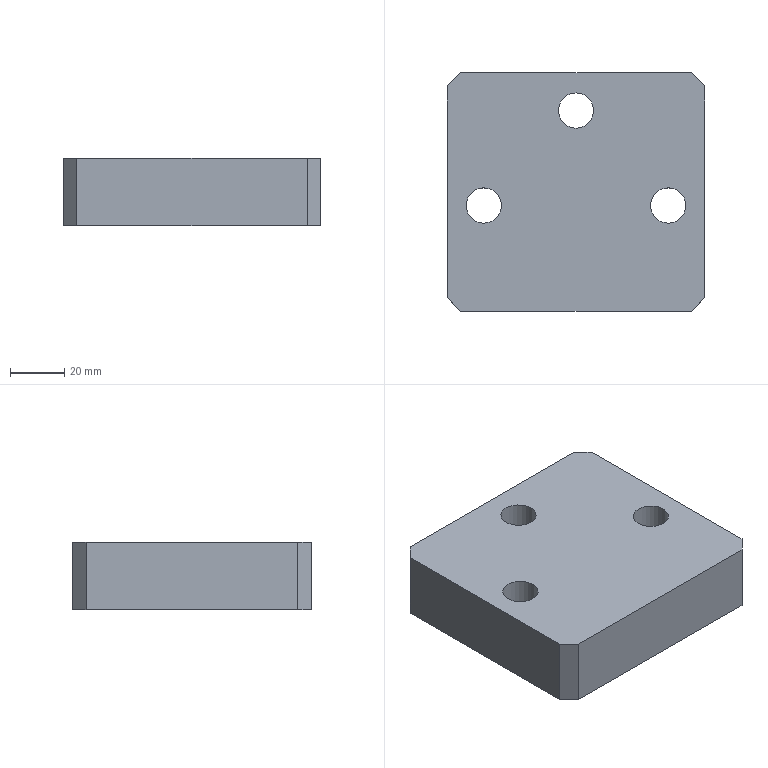Part | STEP file | gslz 2016.10.28-10_id2130_x_t | 1 solid | 19 faces | box 95 x 88 x 25 mm | volume 189649 mm3 | plane 13 | cylinder 6 | commonest cylinder face diameters 13 x3 20 x3
STEP:
#1=CARTESIAN_POINT('',(0.,0.,0.));
#2=DIRECTION('',(0.,0.,1.));
#3=DIRECTION('',(1.,0.,0.));
#4=AXIS2_PLACEMENT_3D('',#1,#2,#3);
#5=CARTESIAN_POINT('',(589.,313.071,3.));
#6=VERTEX_POINT('',#5);
#7=CARTESIAN_POINT('',(589.,235.,3.));
#8=VERTEX_POINT('',#7);
#9=CARTESIAN_POINT('',(589.,-635.206,3.));
#10=DIRECTION('',(0.,-1.,0.));
#11=VECTOR('',#10,1.);
#12=LINE('',#9,#11);
#13=CARTESIAN_POINT('',(589.,-627.983,-1.));
#14=DIRECTION('',(-1.,0.,0.));
#15=DIRECTION('',(0.,0.,1.));
#16=AXIS2_PLACEMENT_3D('',#13,#14,#15);
#17=PLANE('',#16);
#18=CARTESIAN_POINT('',(4.,-7.223));
#19=DIRECTION('',(0.,-1.));
#20=VECTOR('',#19,1.);
#21=LINE('',#18,#20);
#22=(GEOMETRIC_REPRESENTATION_CONTEXT(2)PARAMETRIC_REPRESENTATION_CONTEXT()REPRESENTATION_CONTEXT('',''));
#23=DEFINITIONAL_REPRESENTATION('',(#21),#22);
#24=PCURVE('',#17,#23);
#25=CARTESIAN_POINT('',(-3.966,-635.206,3.));
#26=DIRECTION('',(0.,0.,1.));
#27=DIRECTION('',(1.,0.,0.));
#28=AXIS2_PLACEMENT_3D('',#25,#26,#27);
#29=PLANE('',#28);
#30=CARTESIAN_POINT('',(592.966,0.));
#31=DIRECTION('',(0.,-1.));
#32=VECTOR('',#31,1.);
#33=LINE('',#30,#32);
#34=(GEOMETRIC_REPRESENTATION_CONTEXT(2)PARAMETRIC_REPRESENTATION_CONTEXT()REPRESENTATION_CONTEXT('',''));
#35=DEFINITIONAL_REPRESENTATION('',(#33),#34);
#36=PCURVE('',#29,#35);
#37=SURFACE_CURVE('',#12,(#24,#36),.PCURVE_S1.);
#38=EDGE_CURVE('',#6,#8,#37,.T.);
#39=ORIENTED_EDGE('',*,*,#38,.F.);
#40=CARTESIAN_POINT('',(589.,313.071,-22.));
#41=VERTEX_POINT('',#40);
#42=CARTESIAN_POINT('',(589.,313.071,-1.));
#43=DIRECTION('',(0.,0.,-1.));
#44=VECTOR('',#43,1.);
#45=LINE('',#42,#44);
#46=CARTESIAN_POINT('',(0.,941.054));
#47=DIRECTION('',(-1.,0.));
#48=VECTOR('',#47,1.);
#49=LINE('',#46,#48);
#50=(GEOMETRIC_REPRESENTATION_CONTEXT(2)PARAMETRIC_REPRESENTATION_CONTEXT()REPRESENTATION_CONTEXT('',''));
#51=DEFINITIONAL_REPRESENTATION('',(#49),#50);
#52=PCURVE('',#17,#51);
#53=CARTESIAN_POINT('',(592.464,316.536,49.));
#54=DIRECTION('',(0.7071,-0.7071,0.));
#55=DIRECTION('',(0.,0.,1.));
#56=AXIS2_PLACEMENT_3D('',#53,#54,#55);
#57=PLANE('',#56);
#58=CARTESIAN_POINT('',(-50.,4.899));
#59=DIRECTION('',(-1.,0.));
#60=VECTOR('',#59,1.);
#61=LINE('',#58,#60);
#62=(GEOMETRIC_REPRESENTATION_CONTEXT(2)PARAMETRIC_REPRESENTATION_CONTEXT()REPRESENTATION_CONTEXT('',''));
#63=DEFINITIONAL_REPRESENTATION('',(#61),#62);
#64=PCURVE('',#57,#63);
#65=SURFACE_CURVE('',#45,(#52,#64),.PCURVE_S1.);
#66=EDGE_CURVE('',#6,#41,#65,.T.);
#67=ORIENTED_EDGE('',*,*,#66,.T.);
#68=CARTESIAN_POINT('',(589.,235.,-22.));
#69=VERTEX_POINT('',#68);
#70=CARTESIAN_POINT('',(589.,-635.206,-22.));
#71=DIRECTION('',(0.,-1.,0.));
#72=VECTOR('',#71,1.);
#73=LINE('',#70,#72);
#74=CARTESIAN_POINT('',(-21.,-7.223));
#75=DIRECTION('',(0.,-1.));
#76=VECTOR('',#75,1.);
#77=LINE('',#74,#76);
#78=(GEOMETRIC_REPRESENTATION_CONTEXT(2)PARAMETRIC_REPRESENTATION_CONTEXT()REPRESENTATION_CONTEXT('',''));
#79=DEFINITIONAL_REPRESENTATION('',(#77),#78);
#80=PCURVE('',#17,#79);
#81=CARTESIAN_POINT('',(-3.966,-635.206,-22.));
#82=DIRECTION('',(0.,0.,1.));
#83=DIRECTION('',(1.,0.,0.));
#84=AXIS2_PLACEMENT_3D('',#81,#82,#83);
#85=PLANE('',#84);
#86=CARTESIAN_POINT('',(592.966,0.));
#87=DIRECTION('',(0.,-1.));
#88=VECTOR('',#87,1.);
#89=LINE('',#86,#88);
#90=(GEOMETRIC_REPRESENTATION_CONTEXT(2)PARAMETRIC_REPRESENTATION_CONTEXT()REPRESENTATION_CONTEXT('',''));
#91=DEFINITIONAL_REPRESENTATION('',(#89),#90);
#92=PCURVE('',#85,#91);
#93=SURFACE_CURVE('',#73,(#80,#92),.PCURVE_S1.);
#94=EDGE_CURVE('',#41,#69,#93,.T.);
#95=ORIENTED_EDGE('',*,*,#94,.T.);
#96=CARTESIAN_POINT('',(589.,235.,-17.));
#97=DIRECTION('',(0.,0.,1.));
#98=VECTOR('',#97,1.);
#99=LINE('',#96,#98);
#100=CARTESIAN_POINT('',(-16.,862.983));
#101=DIRECTION('',(1.,0.));
#102=VECTOR('',#101,1.);
#103=LINE('',#100,#102);
#104=(GEOMETRIC_REPRESENTATION_CONTEXT(2)PARAMETRIC_REPRESENTATION_CONTEXT()REPRESENTATION_CONTEXT('',''));
#105=DEFINITIONAL_REPRESENTATION('',(#103),#104);
#106=PCURVE('',#17,#105);
#107=CARTESIAN_POINT('',(589.,235.,-1.));
#108=DIRECTION('',(0.7071,0.7071,0.));
#109=DIRECTION('',(0.,0.,1.));
#110=AXIS2_PLACEMENT_3D('',#107,#108,#109);
#111=PLANE('',#110);
#112=CARTESIAN_POINT('',(-16.,0.));
#113=DIRECTION('',(1.,0.));
#114=VECTOR('',#113,1.);
#115=LINE('',#112,#114);
#116=(GEOMETRIC_REPRESENTATION_CONTEXT(2)PARAMETRIC_REPRESENTATION_CONTEXT()REPRESENTATION_CONTEXT('',''));
#117=DEFINITIONAL_REPRESENTATION('',(#115),#116);
#118=PCURVE('',#111,#117);
#119=SURFACE_CURVE('',#99,(#106,#118),.PCURVE_S1.);
#120=EDGE_CURVE('',#69,#8,#119,.T.);
#121=ORIENTED_EDGE('',*,*,#120,.T.);
#122=EDGE_LOOP('',(#39,#67,#95,#121));
#123=FACE_BOUND('',#122,.T.);
#124=ADVANCED_FACE('',(#123),#17,.T.);
#125=CARTESIAN_POINT('',(684.,235.,-22.));
#126=VERTEX_POINT('',#125);
#127=CARTESIAN_POINT('',(684.,313.071,-22.));
#128=VERTEX_POINT('',#127);
#129=CARTESIAN_POINT('',(684.,-635.206,-22.));
#130=DIRECTION('',(0.,1.,0.));
#131=VECTOR('',#130,1.);
#132=LINE('',#129,#131);
#133=CARTESIAN_POINT('',(684.,-627.983,-1.));
#134=DIRECTION('',(1.,0.,0.));
#135=DIRECTION('',(0.,0.,-1.));
#136=AXIS2_PLACEMENT_3D('',#133,#134,#135);
#137=PLANE('',#136);
#138=CARTESIAN_POINT('',(21.,-7.223));
#139=DIRECTION('',(0.,1.));
#140=VECTOR('',#139,1.);
#141=LINE('',#138,#140);
#142=(GEOMETRIC_REPRESENTATION_CONTEXT(2)PARAMETRIC_REPRESENTATION_CONTEXT()REPRESENTATION_CONTEXT('',''));
#143=DEFINITIONAL_REPRESENTATION('',(#141),#142);
#144=PCURVE('',#137,#143);
#145=CARTESIAN_POINT('',(687.966,0.));
#146=DIRECTION('',(0.,1.));
#147=VECTOR('',#146,1.);
#148=LINE('',#145,#147);
#149=(GEOMETRIC_REPRESENTATION_CONTEXT(2)PARAMETRIC_REPRESENTATION_CONTEXT()REPRESENTATION_CONTEXT('',''));
#150=DEFINITIONAL_REPRESENTATION('',(#148),#149);
#151=PCURVE('',#85,#150);
#152=SURFACE_CURVE('',#132,(#144,#151),.PCURVE_S1.);
#153=EDGE_CURVE('',#126,#128,#152,.T.);
#154=ORIENTED_EDGE('',*,*,#153,.T.);
#155=CARTESIAN_POINT('',(684.,313.071,3.));
#156=VERTEX_POINT('',#155);
#157=CARTESIAN_POINT('',(684.,313.071,-1.));
#158=DIRECTION('',(0.,0.,1.));
#159=VECTOR('',#158,1.);
#160=LINE('',#157,#159);
#161=CARTESIAN_POINT('',(0.,941.054));
#162=DIRECTION('',(-1.,0.));
#163=VECTOR('',#162,1.);
#164=LINE('',#161,#163);
#165=(GEOMETRIC_REPRESENTATION_CONTEXT(2)PARAMETRIC_REPRESENTATION_CONTEXT()REPRESENTATION_CONTEXT('',''));
#166=DEFINITIONAL_REPRESENTATION('',(#164),#165);
#167=PCURVE('',#137,#166);
#168=CARTESIAN_POINT('',(682.536,314.536,-1.));
#169=DIRECTION('',(-0.7071,-0.7071,0.));
#170=DIRECTION('',(0.,0.,1.));
#171=AXIS2_PLACEMENT_3D('',#168,#169,#170);
#172=PLANE('',#171);
#173=CARTESIAN_POINT('',(0.,-2.071));
#174=DIRECTION('',(1.,0.));
#175=VECTOR('',#174,1.);
#176=LINE('',#173,#175);
#177=(GEOMETRIC_REPRESENTATION_CONTEXT(2)PARAMETRIC_REPRESENTATION_CONTEXT()REPRESENTATION_CONTEXT('',''));
#178=DEFINITIONAL_REPRESENTATION('',(#176),#177);
#179=PCURVE('',#172,#178);
#180=SURFACE_CURVE('',#160,(#167,#179),.PCURVE_S1.);
#181=EDGE_CURVE('',#128,#156,#180,.T.);
#182=ORIENTED_EDGE('',*,*,#181,.T.);
#183=CARTESIAN_POINT('',(684.,235.,3.));
#184=VERTEX_POINT('',#183);
#185=CARTESIAN_POINT('',(684.,-635.206,3.));
#186=DIRECTION('',(0.,1.,0.));
#187=VECTOR('',#186,1.);
#188=LINE('',#185,#187);
#189=CARTESIAN_POINT('',(-4.,-7.223));
#190=DIRECTION('',(0.,1.));
#191=VECTOR('',#190,1.);
#192=LINE('',#189,#191);
#193=(GEOMETRIC_REPRESENTATION_CONTEXT(2)PARAMETRIC_REPRESENTATION_CONTEXT()REPRESENTATION_CONTEXT('',''));
#194=DEFINITIONAL_REPRESENTATION('',(#192),#193);
#195=PCURVE('',#137,#194);
#196=CARTESIAN_POINT('',(687.966,0.));
#197=DIRECTION('',(0.,1.));
#198=VECTOR('',#197,1.);
#199=LINE('',#196,#198);
#200=(GEOMETRIC_REPRESENTATION_CONTEXT(2)PARAMETRIC_REPRESENTATION_CONTEXT()REPRESENTATION_CONTEXT('',''));
#201=DEFINITIONAL_REPRESENTATION('',(#199),#200);
#202=PCURVE('',#29,#201);
#203=SURFACE_CURVE('',#188,(#195,#202),.PCURVE_S1.);
#204=EDGE_CURVE('',#184,#156,#203,.T.);
#205=ORIENTED_EDGE('',*,*,#204,.F.);
#206=CARTESIAN_POINT('',(684.,235.,3.));
#207=DIRECTION('',(0.,0.,-1.));
#208=VECTOR('',#207,1.);
#209=LINE('',#206,#208);
#210=CARTESIAN_POINT('',(-4.,862.983));
#211=DIRECTION('',(1.,0.));
#212=VECTOR('',#211,1.);
#213=LINE('',#210,#212);
#214=(GEOMETRIC_REPRESENTATION_CONTEXT(2)PARAMETRIC_REPRESENTATION_CONTEXT()REPRESENTATION_CONTEXT('',''));
#215=DEFINITIONAL_REPRESENTATION('',(#213),#214);
#216=PCURVE('',#137,#215);
#217=CARTESIAN_POINT('',(679.,230.,4.));
#218=DIRECTION('',(-0.7071,0.7071,0.));
#219=DIRECTION('',(0.,0.,1.));
#220=AXIS2_PLACEMENT_3D('',#217,#218,#219);
#221=PLANE('',#220);
#222=CARTESIAN_POINT('',(-1.,7.071));
#223=DIRECTION('',(-1.,0.));
#224=VECTOR('',#223,1.);
#225=LINE('',#222,#224);
#226=(GEOMETRIC_REPRESENTATION_CONTEXT(2)PARAMETRIC_REPRESENTATION_CONTEXT()REPRESENTATION_CONTEXT('',''));
#227=DEFINITIONAL_REPRESENTATION('',(#225),#226);
#228=PCURVE('',#221,#227);
#229=SURFACE_CURVE('',#209,(#216,#228),.PCURVE_S1.);
#230=EDGE_CURVE('',#184,#126,#229,.T.);
#231=ORIENTED_EDGE('',*,*,#230,.T.);
#232=EDGE_LOOP('',(#154,#182,#205,#231));
#233=FACE_BOUND('',#232,.T.);
#234=ADVANCED_FACE('',(#233),#137,.T.);
#235=CARTESIAN_POINT('',(636.5,314.,-22.));
#236=VERTEX_POINT('',#235);
#237=CARTESIAN_POINT('',(636.5,294.,-22.));
#238=VERTEX_POINT('',#237);
#239=CARTESIAN_POINT('',(636.5,304.,-22.));
#240=DIRECTION('',(0.,0.,1.));
#241=DIRECTION('',(0.,1.,0.));
#242=AXIS2_PLACEMENT_3D('',#239,#240,#241);
#243=CIRCLE('',#242,10.);
#244=CARTESIAN_POINT('',(640.466,939.206));
#245=DIRECTION('',(0.,1.));
#246=AXIS2_PLACEMENT_2D('',#244,#245);
#247=CIRCLE('',#246,10.);
#248=(GEOMETRIC_REPRESENTATION_CONTEXT(2)PARAMETRIC_REPRESENTATION_CONTEXT()REPRESENTATION_CONTEXT('',''));
#249=DEFINITIONAL_REPRESENTATION('',(#247),#248);
#250=PCURVE('',#85,#249);
#251=CARTESIAN_POINT('',(636.5,304.,3.));
#252=DIRECTION('',(0.,0.,1.));
#253=DIRECTION('',(1.,0.,0.));
#254=AXIS2_PLACEMENT_3D('',#251,#252,#253);
#255=CYLINDRICAL_SURFACE('',#254,10.);
#256=CARTESIAN_POINT('',(7.854,-25.));
#257=DIRECTION('',(1.,0.));
#258=VECTOR('',#257,1.);
#259=LINE('',#256,#258);
#260=(GEOMETRIC_REPRESENTATION_CONTEXT(2)PARAMETRIC_REPRESENTATION_CONTEXT()REPRESENTATION_CONTEXT('',''));
#261=DEFINITIONAL_REPRESENTATION('',(#259),#260);
#262=PCURVE('',#255,#261);
#263=SURFACE_CURVE('',#243,(#250,#262),.PCURVE_S1.);
#264=EDGE_CURVE('',#236,#238,#263,.T.);
#265=ORIENTED_EDGE('',*,*,#264,.T.);
#266=CARTESIAN_POINT('',(636.5,304.,-22.));
#267=DIRECTION('',(0.,0.,1.));
#268=DIRECTION('',(0.,1.,0.));
#269=AXIS2_PLACEMENT_3D('',#266,#267,#268);
#270=CIRCLE('',#269,10.);
#271=CARTESIAN_POINT('',(640.466,939.206));
#272=DIRECTION('',(0.,1.));
#273=AXIS2_PLACEMENT_2D('',#271,#272);
#274=CIRCLE('',#273,10.);
#275=(GEOMETRIC_REPRESENTATION_CONTEXT(2)PARAMETRIC_REPRESENTATION_CONTEXT()REPRESENTATION_CONTEXT('',''));
#276=DEFINITIONAL_REPRESENTATION('',(#274),#275);
#277=PCURVE('',#85,#276);
#278=CARTESIAN_POINT('',(1.571,-25.));
#279=DIRECTION('',(1.,0.));
#280=VECTOR('',#279,1.);
#281=LINE('',#278,#280);
#282=(GEOMETRIC_REPRESENTATION_CONTEXT(2)PARAMETRIC_REPRESENTATION_CONTEXT()REPRESENTATION_CONTEXT('',''));
#283=DEFINITIONAL_REPRESENTATION('',(#281),#282);
#284=PCURVE('',#255,#283);
#285=SURFACE_CURVE('',#270,(#277,#284),.PCURVE_S1.);
#286=EDGE_CURVE('',#238,#236,#285,.T.);
#287=ORIENTED_EDGE('',*,*,#286,.T.);
#288=EDGE_LOOP('',(#265,#287));
#289=FACE_BOUND('',#288,.T.);
#290=CARTESIAN_POINT('',(602.5,279.,-22.));
#291=VERTEX_POINT('',#290);
#292=CARTESIAN_POINT('',(602.5,259.,-22.));
#293=VERTEX_POINT('',#292);
#294=CARTESIAN_POINT('',(602.5,269.,-22.));
#295=DIRECTION('',(0.,0.,-1.));
#296=DIRECTION('',(0.,1.,0.));
#297=AXIS2_PLACEMENT_3D('',#294,#295,#296);
#298=CIRCLE('',#297,10.);
#299=CARTESIAN_POINT('',(606.466,914.206));
#300=CARTESIAN_POINT('',(623.787,914.206));
#301=CARTESIAN_POINT('',(615.127,899.206));
#302=CARTESIAN_POINT('',(606.466,884.206));
#303=CARTESIAN_POINT('',(597.806,899.206));
#304=CARTESIAN_POINT('',(589.146,914.206));
#305=CARTESIAN_POINT('',(606.466,914.206));
#306=(BOUNDED_CURVE()B_SPLINE_CURVE(2,(#299,#300,#301,#302,#303,#304,#305),.UNSPECIFIED.,.T.,.F.)B_SPLINE_CURVE_WITH_KNOTS((1,2,2,2,2,1),(-2.094,0.,2.094,4.189,6.283,8.378),.UNSPECIFIED.)CURVE()GEOMETRIC_REPRESENTATION_ITEM()RATIONAL_B_SPLINE_CURVE((1.,0.5,1.,0.5,1.,0.5,1.))REPRESENTATION_ITEM(''));
#307=(GEOMETRIC_REPRESENTATION_CONTEXT(2)PARAMETRIC_REPRESENTATION_CONTEXT()REPRESENTATION_CONTEXT('',''));
#308=DEFINITIONAL_REPRESENTATION('',(#306),#307);
#309=PCURVE('',#85,#308);
#310=CARTESIAN_POINT('',(602.5,269.,3.));
#311=DIRECTION('',(0.,0.,1.));
#312=DIRECTION('',(1.,0.,0.));
#313=AXIS2_PLACEMENT_3D('',#310,#311,#312);
#314=CYLINDRICAL_SURFACE('',#313,10.);
#315=CARTESIAN_POINT('',(7.854,-25.));
#316=DIRECTION('',(-1.,0.));
#317=VECTOR('',#316,1.);
#318=LINE('',#315,#317);
#319=(GEOMETRIC_REPRESENTATION_CONTEXT(2)PARAMETRIC_REPRESENTATION_CONTEXT()REPRESENTATION_CONTEXT('',''));
#320=DEFINITIONAL_REPRESENTATION('',(#318),#319);
#321=PCURVE('',#314,#320);
#322=SURFACE_CURVE('',#298,(#309,#321),.PCURVE_S1.);
#323=EDGE_CURVE('',#291,#293,#322,.T.);
#324=ORIENTED_EDGE('',*,*,#323,.F.);
#325=CARTESIAN_POINT('',(602.5,269.,-22.));
#326=DIRECTION('',(0.,0.,-1.));
#327=DIRECTION('',(0.,1.,0.));
#328=AXIS2_PLACEMENT_3D('',#325,#326,#327);
#329=CIRCLE('',#328,10.);
#330=CARTESIAN_POINT('',(606.466,914.206));
#331=CARTESIAN_POINT('',(623.787,914.206));
#332=CARTESIAN_POINT('',(615.127,899.206));
#333=CARTESIAN_POINT('',(606.466,884.206));
#334=CARTESIAN_POINT('',(597.806,899.206));
#335=CARTESIAN_POINT('',(589.146,914.206));
#336=CARTESIAN_POINT('',(606.466,914.206));
#337=(BOUNDED_CURVE()B_SPLINE_CURVE(2,(#330,#331,#332,#333,#334,#335,#336),.UNSPECIFIED.,.T.,.F.)B_SPLINE_CURVE_WITH_KNOTS((1,2,2,2,2,1),(-2.094,0.,2.094,4.189,6.283,8.378),.UNSPECIFIED.)CURVE()GEOMETRIC_REPRESENTATION_ITEM()RATIONAL_B_SPLINE_CURVE((1.,0.5,1.,0.5,1.,0.5,1.))REPRESENTATION_ITEM(''));
#338=(GEOMETRIC_REPRESENTATION_CONTEXT(2)PARAMETRIC_REPRESENTATION_CONTEXT()REPRESENTATION_CONTEXT('',''));
#339=DEFINITIONAL_REPRESENTATION('',(#337),#338);
#340=PCURVE('',#85,#339);
#341=CARTESIAN_POINT('',(14.137,-25.));
#342=DIRECTION('',(-1.,0.));
#343=VECTOR('',#342,1.);
#344=LINE('',#341,#343);
#345=(GEOMETRIC_REPRESENTATION_CONTEXT(2)PARAMETRIC_REPRESENTATION_CONTEXT()REPRESENTATION_CONTEXT('',''));
#346=DEFINITIONAL_REPRESENTATION('',(#344),#345);
#347=PCURVE('',#314,#346);
#348=SURFACE_CURVE('',#329,(#340,#347),.PCURVE_S1.);
#349=EDGE_CURVE('',#293,#291,#348,.T.);
#350=ORIENTED_EDGE('',*,*,#349,.F.);
#351=EDGE_LOOP('',(#324,#350));
#352=FACE_BOUND('',#351,.T.);
#353=CARTESIAN_POINT('',(670.5,279.,-22.));
#354=VERTEX_POINT('',#353);
#355=CARTESIAN_POINT('',(670.5,259.,-22.));
#356=VERTEX_POINT('',#355);
#357=CARTESIAN_POINT('',(670.5,269.,-22.));
#358=DIRECTION('',(0.,0.,-1.));
#359=DIRECTION('',(0.,1.,0.));
#360=AXIS2_PLACEMENT_3D('',#357,#358,#359);
#361=CIRCLE('',#360,10.);
#362=CARTESIAN_POINT('',(674.466,914.206));
#363=CARTESIAN_POINT('',(691.787,914.206));
#364=CARTESIAN_POINT('',(683.127,899.206));
#365=CARTESIAN_POINT('',(674.466,884.206));
#366=CARTESIAN_POINT('',(665.806,899.206));
#367=CARTESIAN_POINT('',(657.146,914.206));
#368=CARTESIAN_POINT('',(674.466,914.206));
#369=(BOUNDED_CURVE()B_SPLINE_CURVE(2,(#362,#363,#364,#365,#366,#367,#368),.UNSPECIFIED.,.T.,.F.)B_SPLINE_CURVE_WITH_KNOTS((1,2,2,2,2,1),(-2.094,0.,2.094,4.189,6.283,8.378),.UNSPECIFIED.)CURVE()GEOMETRIC_REPRESENTATION_ITEM()RATIONAL_B_SPLINE_CURVE((1.,0.5,1.,0.5,1.,0.5,1.))REPRESENTATION_ITEM(''));
#370=(GEOMETRIC_REPRESENTATION_CONTEXT(2)PARAMETRIC_REPRESENTATION_CONTEXT()REPRESENTATION_CONTEXT('',''));
#371=DEFINITIONAL_REPRESENTATION('',(#369),#370);
#372=PCURVE('',#85,#371);
#373=CARTESIAN_POINT('',(670.5,269.,3.));
#374=DIRECTION('',(0.,0.,1.));
#375=DIRECTION('',(1.,0.,0.));
#376=AXIS2_PLACEMENT_3D('',#373,#374,#375);
#377=CYLINDRICAL_SURFACE('',#376,10.);
#378=CARTESIAN_POINT('',(7.854,-25.));
#379=DIRECTION('',(-1.,0.));
#380=VECTOR('',#379,1.);
#381=LINE('',#378,#380);
#382=(GEOMETRIC_REPRESENTATION_CONTEXT(2)PARAMETRIC_REPRESENTATION_CONTEXT()REPRESENTATION_CONTEXT('',''));
#383=DEFINITIONAL_REPRESENTATION('',(#381),#382);
#384=PCURVE('',#377,#383);
#385=SURFACE_CURVE('',#361,(#372,#384),.PCURVE_S1.);
#386=EDGE_CURVE('',#354,#356,#385,.T.);
#387=ORIENTED_EDGE('',*,*,#386,.F.);
#388=CARTESIAN_POINT('',(670.5,269.,-22.));
#389=DIRECTION('',(0.,0.,-1.));
#390=DIRECTION('',(0.,1.,0.));
#391=AXIS2_PLACEMENT_3D('',#388,#389,#390);
#392=CIRCLE('',#391,10.);
#393=CARTESIAN_POINT('',(674.466,914.206));
#394=CARTESIAN_POINT('',(691.787,914.206));
#395=CARTESIAN_POINT('',(683.127,899.206));
#396=CARTESIAN_POINT('',(674.466,884.206));
#397=CARTESIAN_POINT('',(665.806,899.206));
#398=CARTESIAN_POINT('',(657.146,914.206));
#399=CARTESIAN_POINT('',(674.466,914.206));
#400=(BOUNDED_CURVE()B_SPLINE_CURVE(2,(#393,#394,#395,#396,#397,#398,#399),.UNSPECIFIED.,.T.,.F.)B_SPLINE_CURVE_WITH_KNOTS((1,2,2,2,2,1),(-2.094,0.,2.094,4.189,6.283,8.378),.UNSPECIFIED.)CURVE()GEOMETRIC_REPRESENTATION_ITEM()RATIONAL_B_SPLINE_CURVE((1.,0.5,1.,0.5,1.,0.5,1.))REPRESENTATION_ITEM(''));
#401=(GEOMETRIC_REPRESENTATION_CONTEXT(2)PARAMETRIC_REPRESENTATION_CONTEXT()REPRESENTATION_CONTEXT('',''));
#402=DEFINITIONAL_REPRESENTATION('',(#400),#401);
#403=PCURVE('',#85,#402);
#404=CARTESIAN_POINT('',(14.137,-25.));
#405=DIRECTION('',(-1.,0.));
#406=VECTOR('',#405,1.);
#407=LINE('',#404,#406);
#408=(GEOMETRIC_REPRESENTATION_CONTEXT(2)PARAMETRIC_REPRESENTATION_CONTEXT()REPRESENTATION_CONTEXT('',''));
#409=DEFINITIONAL_REPRESENTATION('',(#407),#408);
#410=PCURVE('',#377,#409);
#411=SURFACE_CURVE('',#392,(#403,#410),.PCURVE_S1.);
#412=EDGE_CURVE('',#356,#354,#411,.T.);
#413=ORIENTED_EDGE('',*,*,#412,.F.);
#414=EDGE_LOOP('',(#387,#413));
#415=FACE_BOUND('',#414,.T.);
#416=CARTESIAN_POINT('',(594.,230.,-22.));
#417=VERTEX_POINT('',#416);
#418=CARTESIAN_POINT('',(679.,230.,-22.));
#419=VERTEX_POINT('',#418);
#420=CARTESIAN_POINT('',(-3.966,230.,-22.));
#421=DIRECTION('',(1.,0.,0.));
#422=VECTOR('',#421,1.);
#423=LINE('',#420,#422);
#424=CARTESIAN_POINT('',(0.,865.206));
#425=DIRECTION('',(1.,0.));
#426=VECTOR('',#425,1.);
#427=LINE('',#424,#426);
#428=(GEOMETRIC_REPRESENTATION_CONTEXT(2)PARAMETRIC_REPRESENTATION_CONTEXT()REPRESENTATION_CONTEXT('',''));
#429=DEFINITIONAL_REPRESENTATION('',(#427),#428);
#430=PCURVE('',#85,#429);
#431=CARTESIAN_POINT('',(-2.035,230.,4.));
#432=DIRECTION('',(0.,-1.,0.));
#433=DIRECTION('',(-1.,0.,0.));
#434=AXIS2_PLACEMENT_3D('',#431,#432,#433);
#435=PLANE('',#434);
#436=CARTESIAN_POINT('',(1.931,26.));
#437=DIRECTION('',(-1.,0.));
#438=VECTOR('',#437,1.);
#439=LINE('',#436,#438);
#440=(GEOMETRIC_REPRESENTATION_CONTEXT(2)PARAMETRIC_REPRESENTATION_CONTEXT()REPRESENTATION_CONTEXT('',''));
#441=DEFINITIONAL_REPRESENTATION('',(#439),#440);
#442=PCURVE('',#435,#441);
#443=SURFACE_CURVE('',#423,(#430,#442),.PCURVE_S1.);
#444=EDGE_CURVE('',#417,#419,#443,.T.);
#445=ORIENTED_EDGE('',*,*,#444,.F.);
#446=CARTESIAN_POINT('',(589.,235.,-22.));
#447=DIRECTION('',(-0.7071,0.7071,0.));
#448=VECTOR('',#447,1.);
#449=LINE('',#446,#448);
#450=CARTESIAN_POINT('',(592.966,870.206));
#451=DIRECTION('',(-0.7071,0.7071));
#452=VECTOR('',#451,1.);
#453=LINE('',#450,#452);
#454=(GEOMETRIC_REPRESENTATION_CONTEXT(2)PARAMETRIC_REPRESENTATION_CONTEXT()REPRESENTATION_CONTEXT('',''));
#455=DEFINITIONAL_REPRESENTATION('',(#453),#454);
#456=PCURVE('',#85,#455);
#457=CARTESIAN_POINT('',(-21.,0.));
#458=DIRECTION('',(0.,-1.));
#459=VECTOR('',#458,1.);
#460=LINE('',#457,#459);
#461=(GEOMETRIC_REPRESENTATION_CONTEXT(2)PARAMETRIC_REPRESENTATION_CONTEXT()REPRESENTATION_CONTEXT('',''));
#462=DEFINITIONAL_REPRESENTATION('',(#460),#461);
#463=PCURVE('',#111,#462);
#464=SURFACE_CURVE('',#449,(#456,#463),.PCURVE_S1.);
#465=EDGE_CURVE('',#417,#69,#464,.T.);
#466=ORIENTED_EDGE('',*,*,#465,.T.);
#467=ORIENTED_EDGE('',*,*,#94,.F.);
#468=CARTESIAN_POINT('',(593.929,318.,-22.));
#469=VERTEX_POINT('',#468);
#470=CARTESIAN_POINT('',(592.464,316.536,-22.));
#471=DIRECTION('',(0.7071,0.7071,0.));
#472=VECTOR('',#471,1.);
#473=LINE('',#470,#472);
#474=CARTESIAN_POINT('',(596.431,951.741));
#475=DIRECTION('',(0.7071,0.7071));
#476=VECTOR('',#475,1.);
#477=LINE('',#474,#476);
#478=(GEOMETRIC_REPRESENTATION_CONTEXT(2)PARAMETRIC_REPRESENTATION_CONTEXT()REPRESENTATION_CONTEXT('',''));
#479=DEFINITIONAL_REPRESENTATION('',(#477),#478);
#480=PCURVE('',#85,#479);
#481=CARTESIAN_POINT('',(-71.,0.));
#482=DIRECTION('',(0.,-1.));
#483=VECTOR('',#482,1.);
#484=LINE('',#481,#483);
#485=(GEOMETRIC_REPRESENTATION_CONTEXT(2)PARAMETRIC_REPRESENTATION_CONTEXT()REPRESENTATION_CONTEXT('',''));
#486=DEFINITIONAL_REPRESENTATION('',(#484),#485);
#487=PCURVE('',#57,#486);
#488=SURFACE_CURVE('',#473,(#480,#487),.PCURVE_S1.);
#489=EDGE_CURVE('',#41,#469,#488,.T.);
#490=ORIENTED_EDGE('',*,*,#489,.T.);
#491=CARTESIAN_POINT('',(679.071,318.,-22.));
#492=VERTEX_POINT('',#491);
#493=CARTESIAN_POINT('',(-3.966,318.,-22.));
#494=DIRECTION('',(-1.,0.,0.));
#495=VECTOR('',#494,1.);
#496=LINE('',#493,#495);
#497=CARTESIAN_POINT('',(0.,953.206));
#498=DIRECTION('',(-1.,0.));
#499=VECTOR('',#498,1.);
#500=LINE('',#497,#499);
#501=(GEOMETRIC_REPRESENTATION_CONTEXT(2)PARAMETRIC_REPRESENTATION_CONTEXT()REPRESENTATION_CONTEXT('',''));
#502=DEFINITIONAL_REPRESENTATION('',(#500),#501);
#503=PCURVE('',#85,#502);
#504=CARTESIAN_POINT('',(636.5,318.,49.));
#505=DIRECTION('',(0.,1.,0.));
#506=DIRECTION('',(0.,0.,1.));
#507=AXIS2_PLACEMENT_3D('',#504,#505,#506);
#508=PLANE('',#507);
#509=CARTESIAN_POINT('',(-71.,-640.466));
#510=DIRECTION('',(0.,-1.));
#511=VECTOR('',#510,1.);
#512=LINE('',#509,#511);
#513=(GEOMETRIC_REPRESENTATION_CONTEXT(2)PARAMETRIC_REPRESENTATION_CONTEXT()REPRESENTATION_CONTEXT('',''));
#514=DEFINITIONAL_REPRESENTATION('',(#512),#513);
#515=PCURVE('',#508,#514);
#516=SURFACE_CURVE('',#496,(#503,#515),.PCURVE_S1.);
#517=EDGE_CURVE('',#492,#469,#516,.T.);
#518=ORIENTED_EDGE('',*,*,#517,.F.);
#519=CARTESIAN_POINT('',(682.536,314.536,-22.));
#520=DIRECTION('',(0.7071,-0.7071,0.));
#521=VECTOR('',#520,1.);
#522=LINE('',#519,#521);
#523=CARTESIAN_POINT('',(686.502,949.741));
#524=DIRECTION('',(0.7071,-0.7071));
#525=VECTOR('',#524,1.);
#526=LINE('',#523,#525);
#527=(GEOMETRIC_REPRESENTATION_CONTEXT(2)PARAMETRIC_REPRESENTATION_CONTEXT()REPRESENTATION_CONTEXT('',''));
#528=DEFINITIONAL_REPRESENTATION('',(#526),#527);
#529=PCURVE('',#85,#528);
#530=CARTESIAN_POINT('',(-21.,0.));
#531=DIRECTION('',(0.,-1.));
#532=VECTOR('',#531,1.);
#533=LINE('',#530,#532);
#534=(GEOMETRIC_REPRESENTATION_CONTEXT(2)PARAMETRIC_REPRESENTATION_CONTEXT()REPRESENTATION_CONTEXT('',''));
#535=DEFINITIONAL_REPRESENTATION('',(#533),#534);
#536=PCURVE('',#172,#535);
#537=SURFACE_CURVE('',#522,(#529,#536),.PCURVE_S1.);
#538=EDGE_CURVE('',#492,#128,#537,.T.);
#539=ORIENTED_EDGE('',*,*,#538,.T.);
#540=ORIENTED_EDGE('',*,*,#153,.F.);
#541=CARTESIAN_POINT('',(679.,230.,-22.));
#542=DIRECTION('',(-0.7071,-0.7071,0.));
#543=VECTOR('',#542,1.);
#544=LINE('',#541,#543);
#545=CARTESIAN_POINT('',(682.966,865.206));
#546=DIRECTION('',(-0.7071,-0.7071));
#547=VECTOR('',#546,1.);
#548=LINE('',#545,#547);
#549=(GEOMETRIC_REPRESENTATION_CONTEXT(2)PARAMETRIC_REPRESENTATION_CONTEXT()REPRESENTATION_CONTEXT('',''));
#550=DEFINITIONAL_REPRESENTATION('',(#548),#549);
#551=PCURVE('',#85,#550);
#552=CARTESIAN_POINT('',(-26.,0.));
#553=DIRECTION('',(0.,-1.));
#554=VECTOR('',#553,1.);
#555=LINE('',#552,#554);
#556=(GEOMETRIC_REPRESENTATION_CONTEXT(2)PARAMETRIC_REPRESENTATION_CONTEXT()REPRESENTATION_CONTEXT('',''));
#557=DEFINITIONAL_REPRESENTATION('',(#555),#556);
#558=PCURVE('',#221,#557);
#559=SURFACE_CURVE('',#544,(#551,#558),.PCURVE_S1.);
#560=EDGE_CURVE('',#126,#419,#559,.T.);
#561=ORIENTED_EDGE('',*,*,#560,.T.);
#562=EDGE_LOOP('',(#445,#466,#467,#490,#518,#539,#540,#561));
#563=FACE_BOUND('',#562,.T.);
#564=ADVANCED_FACE('',(#289,#352,#415,#563),#85,.F.);
#565=CARTESIAN_POINT('',(670.5,275.5,3.));
#566=VERTEX_POINT('',#565);
#567=CARTESIAN_POINT('',(670.5,269.,3.));
#568=DIRECTION('',(0.,0.,1.));
#569=DIRECTION('',(0.,1.,0.));
#570=AXIS2_PLACEMENT_3D('',#567,#568,#569);
#571=CIRCLE('',#570,6.5);
#572=CARTESIAN_POINT('',(674.466,904.206));
#573=DIRECTION('',(0.,1.));
#574=AXIS2_PLACEMENT_2D('',#572,#573);
#575=CIRCLE('',#574,6.5);
#576=(GEOMETRIC_REPRESENTATION_CONTEXT(2)PARAMETRIC_REPRESENTATION_CONTEXT()REPRESENTATION_CONTEXT('',''));
#577=DEFINITIONAL_REPRESENTATION('',(#575),#576);
#578=PCURVE('',#29,#577);
#579=CARTESIAN_POINT('',(670.5,269.,-84.));
#580=DIRECTION('',(0.,0.,1.));
#581=DIRECTION('',(0.,1.,0.));
#582=AXIS2_PLACEMENT_3D('',#579,#580,#581);
#583=CYLINDRICAL_SURFACE('',#582,6.5);
#584=CARTESIAN_POINT('',(0.,87.));
#585=DIRECTION('',(1.,0.));
#586=VECTOR('',#585,1.);
#587=LINE('',#584,#586);
#588=(GEOMETRIC_REPRESENTATION_CONTEXT(2)PARAMETRIC_REPRESENTATION_CONTEXT()REPRESENTATION_CONTEXT('',''));
#589=DEFINITIONAL_REPRESENTATION('',(#587),#588);
#590=PCURVE('',#583,#589);
#591=SURFACE_CURVE('',#571,(#578,#590),.PCURVE_S1.);
#592=EDGE_CURVE('',#566,#566,#591,.T.);
#593=ORIENTED_EDGE('',*,*,#592,.F.);
#594=EDGE_LOOP('',(#593));
#595=FACE_BOUND('',#594,.T.);
#596=CARTESIAN_POINT('',(636.5,310.5,3.));
#597=VERTEX_POINT('',#596);
#598=CARTESIAN_POINT('',(636.5,304.,3.));
#599=DIRECTION('',(0.,0.,1.));
#600=DIRECTION('',(0.,1.,0.));
#601=AXIS2_PLACEMENT_3D('',#598,#599,#600);
#602=CIRCLE('',#601,6.5);
#603=CARTESIAN_POINT('',(640.466,939.206));
#604=DIRECTION('',(0.,1.));
#605=AXIS2_PLACEMENT_2D('',#603,#604);
#606=CIRCLE('',#605,6.5);
#607=(GEOMETRIC_REPRESENTATION_CONTEXT(2)PARAMETRIC_REPRESENTATION_CONTEXT()REPRESENTATION_CONTEXT('',''));
#608=DEFINITIONAL_REPRESENTATION('',(#606),#607);
#609=PCURVE('',#29,#608);
#610=CARTESIAN_POINT('',(636.5,304.,-84.));
#611=DIRECTION('',(0.,0.,1.));
#612=DIRECTION('',(0.,1.,0.));
#613=AXIS2_PLACEMENT_3D('',#610,#611,#612);
#614=CYLINDRICAL_SURFACE('',#613,6.5);
#615=CARTESIAN_POINT('',(0.,87.));
#616=DIRECTION('',(1.,0.));
#617=VECTOR('',#616,1.);
#618=LINE('',#615,#617);
#619=(GEOMETRIC_REPRESENTATION_CONTEXT(2)PARAMETRIC_REPRESENTATION_CONTEXT()REPRESENTATION_CONTEXT('',''));
#620=DEFINITIONAL_REPRESENTATION('',(#618),#619);
#621=PCURVE('',#614,#620);
#622=SURFACE_CURVE('',#602,(#609,#621),.PCURVE_S1.);
#623=EDGE_CURVE('',#597,#597,#622,.T.);
#624=ORIENTED_EDGE('',*,*,#623,.F.);
#625=EDGE_LOOP('',(#624));
#626=FACE_BOUND('',#625,.T.);
#627=CARTESIAN_POINT('',(602.5,275.5,3.));
#628=VERTEX_POINT('',#627);
#629=CARTESIAN_POINT('',(602.5,269.,3.));
#630=DIRECTION('',(0.,0.,1.));
#631=DIRECTION('',(0.,1.,0.));
#632=AXIS2_PLACEMENT_3D('',#629,#630,#631);
#633=CIRCLE('',#632,6.5);
#634=CARTESIAN_POINT('',(606.466,904.206));
#635=DIRECTION('',(0.,1.));
#636=AXIS2_PLACEMENT_2D('',#634,#635);
#637=CIRCLE('',#636,6.5);
#638=(GEOMETRIC_REPRESENTATION_CONTEXT(2)PARAMETRIC_REPRESENTATION_CONTEXT()REPRESENTATION_CONTEXT('',''));
#639=DEFINITIONAL_REPRESENTATION('',(#637),#638);
#640=PCURVE('',#29,#639);
#641=CARTESIAN_POINT('',(602.5,269.,-84.));
#642=DIRECTION('',(0.,0.,1.));
#643=DIRECTION('',(0.,1.,0.));
#644=AXIS2_PLACEMENT_3D('',#641,#642,#643);
#645=CYLINDRICAL_SURFACE('',#644,6.5);
#646=CARTESIAN_POINT('',(0.,87.));
#647=DIRECTION('',(1.,0.));
#648=VECTOR('',#647,1.);
#649=LINE('',#646,#648);
#650=(GEOMETRIC_REPRESENTATION_CONTEXT(2)PARAMETRIC_REPRESENTATION_CONTEXT()REPRESENTATION_CONTEXT('',''));
#651=DEFINITIONAL_REPRESENTATION('',(#649),#650);
#652=PCURVE('',#645,#651);
#653=SURFACE_CURVE('',#633,(#640,#652),.PCURVE_S1.);
#654=EDGE_CURVE('',#628,#628,#653,.T.);
#655=ORIENTED_EDGE('',*,*,#654,.F.);
#656=EDGE_LOOP('',(#655));
#657=FACE_BOUND('',#656,.T.);
#658=ORIENTED_EDGE('',*,*,#204,.T.);
#659=CARTESIAN_POINT('',(679.071,318.,3.));
#660=VERTEX_POINT('',#659);
#661=CARTESIAN_POINT('',(815.155,181.916,3.));
#662=DIRECTION('',(-0.7071,0.7071,0.));
#663=VECTOR('',#662,1.);
#664=LINE('',#661,#663);
#665=CARTESIAN_POINT('',(819.121,817.121));
#666=DIRECTION('',(-0.7071,0.7071));
#667=VECTOR('',#666,1.);
#668=LINE('',#665,#667);
#669=(GEOMETRIC_REPRESENTATION_CONTEXT(2)PARAMETRIC_REPRESENTATION_CONTEXT()REPRESENTATION_CONTEXT('',''));
#670=DEFINITIONAL_REPRESENTATION('',(#668),#669);
#671=PCURVE('',#29,#670);
#672=CARTESIAN_POINT('',(4.,-187.552));
#673=DIRECTION('',(0.,1.));
#674=VECTOR('',#673,1.);
#675=LINE('',#672,#674);
#676=(GEOMETRIC_REPRESENTATION_CONTEXT(2)PARAMETRIC_REPRESENTATION_CONTEXT()REPRESENTATION_CONTEXT('',''));
#677=DEFINITIONAL_REPRESENTATION('',(#675),#676);
#678=PCURVE('',#172,#677);
#679=SURFACE_CURVE('',#664,(#671,#678),.PCURVE_S1.);
#680=EDGE_CURVE('',#156,#660,#679,.T.);
#681=ORIENTED_EDGE('',*,*,#680,.T.);
#682=CARTESIAN_POINT('',(593.929,318.,3.));
#683=VERTEX_POINT('',#682);
#684=CARTESIAN_POINT('',(-3.966,318.,3.));
#685=DIRECTION('',(-1.,0.,0.));
#686=VECTOR('',#685,1.);
#687=LINE('',#684,#686);
#688=CARTESIAN_POINT('',(0.,953.206));
#689=DIRECTION('',(-1.,0.));
#690=VECTOR('',#689,1.);
#691=LINE('',#688,#690);
#692=(GEOMETRIC_REPRESENTATION_CONTEXT(2)PARAMETRIC_REPRESENTATION_CONTEXT()REPRESENTATION_CONTEXT('',''));
#693=DEFINITIONAL_REPRESENTATION('',(#691),#692);
#694=PCURVE('',#29,#693);
#695=CARTESIAN_POINT('',(-46.,-640.466));
#696=DIRECTION('',(0.,-1.));
#697=VECTOR('',#696,1.);
#698=LINE('',#695,#697);
#699=(GEOMETRIC_REPRESENTATION_CONTEXT(2)PARAMETRIC_REPRESENTATION_CONTEXT()REPRESENTATION_CONTEXT('',''));
#700=DEFINITIONAL_REPRESENTATION('',(#698),#699);
#701=PCURVE('',#508,#700);
#702=SURFACE_CURVE('',#687,(#694,#701),.PCURVE_S1.);
#703=EDGE_CURVE('',#660,#683,#702,.T.);
#704=ORIENTED_EDGE('',*,*,#703,.T.);
#705=CARTESIAN_POINT('',(-182.621,-458.55,3.));
#706=DIRECTION('',(-0.7071,-0.7071,0.));
#707=VECTOR('',#706,1.);
#708=LINE('',#705,#707);
#709=CARTESIAN_POINT('',(-178.655,176.655));
#710=DIRECTION('',(-0.7071,-0.7071));
#711=VECTOR('',#710,1.);
#712=LINE('',#709,#711);
#713=(GEOMETRIC_REPRESENTATION_CONTEXT(2)PARAMETRIC_REPRESENTATION_CONTEXT()REPRESENTATION_CONTEXT('',''));
#714=DEFINITIONAL_REPRESENTATION('',(#712),#713);
#715=PCURVE('',#29,#714);
#716=CARTESIAN_POINT('',(-46.,1096.137));
#717=DIRECTION('',(0.,1.));
#718=VECTOR('',#717,1.);
#719=LINE('',#716,#718);
#720=(GEOMETRIC_REPRESENTATION_CONTEXT(2)PARAMETRIC_REPRESENTATION_CONTEXT()REPRESENTATION_CONTEXT('',''));
#721=DEFINITIONAL_REPRESENTATION('',(#719),#720);
#722=PCURVE('',#57,#721);
#723=SURFACE_CURVE('',#708,(#715,#722),.PCURVE_S1.);
#724=EDGE_CURVE('',#683,#6,#723,.T.);
#725=ORIENTED_EDGE('',*,*,#724,.T.);
#726=ORIENTED_EDGE('',*,*,#38,.T.);
#727=CARTESIAN_POINT('',(594.,230.,3.));
#728=VERTEX_POINT('',#727);
#729=CARTESIAN_POINT('',(725.12,98.88,3.));
#730=DIRECTION('',(0.7071,-0.7071,0.));
#731=VECTOR('',#730,1.);
#732=LINE('',#729,#731);
#733=CARTESIAN_POINT('',(729.086,734.086));
#734=DIRECTION('',(0.7071,-0.7071));
#735=VECTOR('',#734,1.);
#736=LINE('',#733,#735);
#737=(GEOMETRIC_REPRESENTATION_CONTEXT(2)PARAMETRIC_REPRESENTATION_CONTEXT()REPRESENTATION_CONTEXT('',''));
#738=DEFINITIONAL_REPRESENTATION('',(#736),#737);
#739=PCURVE('',#29,#738);
#740=CARTESIAN_POINT('',(4.,192.502));
#741=DIRECTION('',(0.,1.));
#742=VECTOR('',#741,1.);
#743=LINE('',#740,#742);
#744=(GEOMETRIC_REPRESENTATION_CONTEXT(2)PARAMETRIC_REPRESENTATION_CONTEXT()REPRESENTATION_CONTEXT('',''));
#745=DEFINITIONAL_REPRESENTATION('',(#743),#744);
#746=PCURVE('',#111,#745);
#747=SURFACE_CURVE('',#732,(#739,#746),.PCURVE_S1.);
#748=EDGE_CURVE('',#8,#728,#747,.T.);
#749=ORIENTED_EDGE('',*,*,#748,.T.);
#750=CARTESIAN_POINT('',(679.,230.,3.));
#751=VERTEX_POINT('',#750);
#752=CARTESIAN_POINT('',(-3.966,230.,3.));
#753=DIRECTION('',(1.,0.,0.));
#754=VECTOR('',#753,1.);
#755=LINE('',#752,#754);
#756=CARTESIAN_POINT('',(0.,865.206));
#757=DIRECTION('',(1.,0.));
#758=VECTOR('',#757,1.);
#759=LINE('',#756,#758);
#760=(GEOMETRIC_REPRESENTATION_CONTEXT(2)PARAMETRIC_REPRESENTATION_CONTEXT()REPRESENTATION_CONTEXT('',''));
#761=DEFINITIONAL_REPRESENTATION('',(#759),#760);
#762=PCURVE('',#29,#761);
#763=CARTESIAN_POINT('',(1.931,1.));
#764=DIRECTION('',(-1.,0.));
#765=VECTOR('',#764,1.);
#766=LINE('',#763,#765);
#767=(GEOMETRIC_REPRESENTATION_CONTEXT(2)PARAMETRIC_REPRESENTATION_CONTEXT()REPRESENTATION_CONTEXT('',''));
#768=DEFINITIONAL_REPRESENTATION('',(#766),#767);
#769=PCURVE('',#435,#768);
#770=SURFACE_CURVE('',#755,(#762,#769),.PCURVE_S1.);
#771=EDGE_CURVE('',#728,#751,#770,.T.);
#772=ORIENTED_EDGE('',*,*,#771,.T.);
#773=CARTESIAN_POINT('',(-92.586,-541.586,3.));
#774=DIRECTION('',(0.7071,0.7071,0.));
#775=VECTOR('',#774,1.);
#776=LINE('',#773,#775);
#777=CARTESIAN_POINT('',(-88.62,93.62));
#778=DIRECTION('',(0.7071,0.7071));
#779=VECTOR('',#778,1.);
#780=LINE('',#777,#779);
#781=(GEOMETRIC_REPRESENTATION_CONTEXT(2)PARAMETRIC_REPRESENTATION_CONTEXT()REPRESENTATION_CONTEXT('',''));
#782=DEFINITIONAL_REPRESENTATION('',(#780),#781);
#783=PCURVE('',#29,#782);
#784=CARTESIAN_POINT('',(-1.,-1091.187));
#785=DIRECTION('',(0.,1.));
#786=VECTOR('',#785,1.);
#787=LINE('',#784,#786);
#788=(GEOMETRIC_REPRESENTATION_CONTEXT(2)PARAMETRIC_REPRESENTATION_CONTEXT()REPRESENTATION_CONTEXT('',''));
#789=DEFINITIONAL_REPRESENTATION('',(#787),#788);
#790=PCURVE('',#221,#789);
#791=SURFACE_CURVE('',#776,(#783,#790),.PCURVE_S1.);
#792=EDGE_CURVE('',#751,#184,#791,.T.);
#793=ORIENTED_EDGE('',*,*,#792,.T.);
#794=EDGE_LOOP('',(#658,#681,#704,#725,#726,#749,#772,#793));
#795=FACE_BOUND('',#794,.T.);
#796=ADVANCED_FACE('',(#595,#626,#657,#795),#29,.T.);
#797=CARTESIAN_POINT('',(670.5,259.,-7.));
#798=VERTEX_POINT('',#797);
#799=CARTESIAN_POINT('',(670.5,269.,-7.));
#800=DIRECTION('',(0.,0.,-1.));
#801=DIRECTION('',(0.,-1.,0.));
#802=AXIS2_PLACEMENT_3D('',#799,#800,#801);
#803=CIRCLE('',#802,10.);
#804=CARTESIAN_POINT('',(670.5,269.,-7.));
#805=DIRECTION('',(0.,0.,-1.));
#806=DIRECTION('',(0.,-1.,0.));
#807=AXIS2_PLACEMENT_3D('',#804,#805,#806);
#808=PLANE('',#807);
#809=CARTESIAN_POINT('',(0.,0.));
#810=DIRECTION('',(1.,0.));
#811=AXIS2_PLACEMENT_2D('',#809,#810);
#812=CIRCLE('',#811,10.);
#813=(GEOMETRIC_REPRESENTATION_CONTEXT(2)PARAMETRIC_REPRESENTATION_CONTEXT()REPRESENTATION_CONTEXT('',''));
#814=DEFINITIONAL_REPRESENTATION('',(#812),#813);
#815=PCURVE('',#808,#814);
#816=CARTESIAN_POINT('',(10.996,-10.));
#817=DIRECTION('',(-1.,0.));
#818=VECTOR('',#817,1.);
#819=LINE('',#816,#818);
#820=(GEOMETRIC_REPRESENTATION_CONTEXT(2)PARAMETRIC_REPRESENTATION_CONTEXT()REPRESENTATION_CONTEXT('',''));
#821=DEFINITIONAL_REPRESENTATION('',(#819),#820);
#822=PCURVE('',#377,#821);
#823=SURFACE_CURVE('',#803,(#815,#822),.PCURVE_S1.);
#824=EDGE_CURVE('',#798,#798,#823,.T.);
#825=ORIENTED_EDGE('',*,*,#824,.T.);
#826=EDGE_LOOP('',(#825));
#827=FACE_BOUND('',#826,.T.);
#828=CARTESIAN_POINT('',(670.5,262.5,-7.));
#829=VERTEX_POINT('',#828);
#830=CARTESIAN_POINT('',(670.5,275.5,-7.));
#831=VERTEX_POINT('',#830);
#832=CARTESIAN_POINT('',(670.5,269.,-7.));
#833=DIRECTION('',(0.,0.,1.));
#834=DIRECTION('',(0.,-1.,0.));
#835=AXIS2_PLACEMENT_3D('',#832,#833,#834);
#836=CIRCLE('',#835,6.5);
#837=CARTESIAN_POINT('',(6.5,0.));
#838=CARTESIAN_POINT('',(6.5,-11.258));
#839=CARTESIAN_POINT('',(-3.25,-5.629));
#840=CARTESIAN_POINT('',(-13.,0.));
#841=CARTESIAN_POINT('',(-3.25,5.629));
#842=CARTESIAN_POINT('',(6.5,11.258));
#843=CARTESIAN_POINT('',(6.5,0.));
#844=(BOUNDED_CURVE()B_SPLINE_CURVE(2,(#837,#838,#839,#840,#841,#842,#843),.UNSPECIFIED.,.T.,.F.)B_SPLINE_CURVE_WITH_KNOTS((1,2,2,2,2,1),(-2.094,0.,2.094,4.189,6.283,8.378),.UNSPECIFIED.)CURVE()GEOMETRIC_REPRESENTATION_ITEM()RATIONAL_B_SPLINE_CURVE((1.,0.5,1.,0.5,1.,0.5,1.))REPRESENTATION_ITEM(''));
#845=(GEOMETRIC_REPRESENTATION_CONTEXT(2)PARAMETRIC_REPRESENTATION_CONTEXT()REPRESENTATION_CONTEXT('',''));
#846=DEFINITIONAL_REPRESENTATION('',(#844),#845);
#847=PCURVE('',#808,#846);
#848=CARTESIAN_POINT('',(3.142,77.));
#849=DIRECTION('',(1.,0.));
#850=VECTOR('',#849,1.);
#851=LINE('',#848,#850);
#852=(GEOMETRIC_REPRESENTATION_CONTEXT(2)PARAMETRIC_REPRESENTATION_CONTEXT()REPRESENTATION_CONTEXT('',''));
#853=DEFINITIONAL_REPRESENTATION('',(#851),#852);
#854=PCURVE('',#583,#853);
#855=SURFACE_CURVE('',#836,(#847,#854),.PCURVE_S1.);
#856=EDGE_CURVE('',#829,#831,#855,.T.);
#857=ORIENTED_EDGE('',*,*,#856,.T.);
#858=CARTESIAN_POINT('',(670.5,269.,-7.));
#859=DIRECTION('',(0.,0.,1.));
#860=DIRECTION('',(0.,-1.,0.));
#861=AXIS2_PLACEMENT_3D('',#858,#859,#860);
#862=CIRCLE('',#861,6.5);
#863=CARTESIAN_POINT('',(6.5,0.));
#864=CARTESIAN_POINT('',(6.5,-11.258));
#865=CARTESIAN_POINT('',(-3.25,-5.629));
#866=CARTESIAN_POINT('',(-13.,0.));
#867=CARTESIAN_POINT('',(-3.25,5.629));
#868=CARTESIAN_POINT('',(6.5,11.258));
#869=CARTESIAN_POINT('',(6.5,0.));
#870=(BOUNDED_CURVE()B_SPLINE_CURVE(2,(#863,#864,#865,#866,#867,#868,#869),.UNSPECIFIED.,.T.,.F.)B_SPLINE_CURVE_WITH_KNOTS((1,2,2,2,2,1),(-2.094,0.,2.094,4.189,6.283,8.378),.UNSPECIFIED.)CURVE()GEOMETRIC_REPRESENTATION_ITEM()RATIONAL_B_SPLINE_CURVE((1.,0.5,1.,0.5,1.,0.5,1.))REPRESENTATION_ITEM(''));
#871=(GEOMETRIC_REPRESENTATION_CONTEXT(2)PARAMETRIC_REPRESENTATION_CONTEXT()REPRESENTATION_CONTEXT('',''));
#872=DEFINITIONAL_REPRESENTATION('',(#870),#871);
#873=PCURVE('',#808,#872);
#874=CARTESIAN_POINT('',(-3.142,77.));
#875=DIRECTION('',(1.,0.));
#876=VECTOR('',#875,1.);
#877=LINE('',#874,#876);
#878=(GEOMETRIC_REPRESENTATION_CONTEXT(2)PARAMETRIC_REPRESENTATION_CONTEXT()REPRESENTATION_CONTEXT('',''));
#879=DEFINITIONAL_REPRESENTATION('',(#877),#878);
#880=PCURVE('',#583,#879);
#881=SURFACE_CURVE('',#862,(#873,#880),.PCURVE_S1.);
#882=EDGE_CURVE('',#831,#829,#881,.T.);
#883=ORIENTED_EDGE('',*,*,#882,.T.);
#884=EDGE_LOOP('',(#857,#883));
#885=FACE_BOUND('',#884,.T.);
#886=ADVANCED_FACE('',(#827,#885),#808,.T.);
#887=ORIENTED_EDGE('',*,*,#824,.T.);
#888=CARTESIAN_POINT('',(670.5,259.,-22.));
#889=CARTESIAN_POINT('',(670.5,259.,-7.));
#890=B_SPLINE_CURVE_WITH_KNOTS('',1,(#888,#889),.UNSPECIFIED.,.F.,.F.,(2,2),(-25.,-10.),.PIECEWISE_BEZIER_KNOTS.);
#891=CARTESIAN_POINT('',(4.712,0.));
#892=DIRECTION('',(0.,1.));
#893=VECTOR('',#892,1.);
#894=LINE('',#891,#893);
#895=(GEOMETRIC_REPRESENTATION_CONTEXT(2)PARAMETRIC_REPRESENTATION_CONTEXT()REPRESENTATION_CONTEXT('',''));
#896=DEFINITIONAL_REPRESENTATION('',(#894),#895);
#897=PCURVE('',#377,#896);
#898=CARTESIAN_POINT('',(10.996,0.));
#899=DIRECTION('',(0.,1.));
#900=VECTOR('',#899,1.);
#901=LINE('',#898,#900);
#902=(GEOMETRIC_REPRESENTATION_CONTEXT(2)PARAMETRIC_REPRESENTATION_CONTEXT()REPRESENTATION_CONTEXT('',''));
#903=DEFINITIONAL_REPRESENTATION('',(#901),#902);
#904=PCURVE('',#377,#903);
#905=SEAM_CURVE('',#890,(#897,#904),.PCURVE_S1.);
#906=EDGE_CURVE('',#356,#798,#905,.T.);
#907=ORIENTED_EDGE('',*,*,#906,.F.);
#908=ORIENTED_EDGE('',*,*,#386,.F.);
#909=ORIENTED_EDGE('',*,*,#412,.F.);
#910=ORIENTED_EDGE('',*,*,#906,.T.);
#911=EDGE_LOOP('',(#887,#907,#908,#909,#910));
#912=FACE_BOUND('',#911,.F.);
#913=ADVANCED_FACE('',(#912),#377,.F.);
#914=ORIENTED_EDGE('',*,*,#592,.F.);
#915=CARTESIAN_POINT('',(670.5,275.5,-7.));
#916=CARTESIAN_POINT('',(670.5,275.5,3.));
#917=B_SPLINE_CURVE_WITH_KNOTS('',1,(#915,#916),.UNSPECIFIED.,.F.,.F.,(2,2),(77.,87.),.PIECEWISE_BEZIER_KNOTS.);
#918=CARTESIAN_POINT('',(0.,0.));
#919=DIRECTION('',(0.,1.));
#920=VECTOR('',#919,1.);
#921=LINE('',#918,#920);
#922=(GEOMETRIC_REPRESENTATION_CONTEXT(2)PARAMETRIC_REPRESENTATION_CONTEXT()REPRESENTATION_CONTEXT('',''));
#923=DEFINITIONAL_REPRESENTATION('',(#921),#922);
#924=PCURVE('',#583,#923);
#925=CARTESIAN_POINT('',(6.283,0.));
#926=DIRECTION('',(0.,1.));
#927=VECTOR('',#926,1.);
#928=LINE('',#925,#927);
#929=(GEOMETRIC_REPRESENTATION_CONTEXT(2)PARAMETRIC_REPRESENTATION_CONTEXT()REPRESENTATION_CONTEXT('',''));
#930=DEFINITIONAL_REPRESENTATION('',(#928),#929);
#931=PCURVE('',#583,#930);
#932=SEAM_CURVE('',#917,(#924,#931),.PCURVE_S1.);
#933=EDGE_CURVE('',#831,#566,#932,.T.);
#934=ORIENTED_EDGE('',*,*,#933,.F.);
#935=ORIENTED_EDGE('',*,*,#882,.T.);
#936=ORIENTED_EDGE('',*,*,#856,.T.);
#937=ORIENTED_EDGE('',*,*,#933,.T.);
#938=EDGE_LOOP('',(#914,#934,#935,#936,#937));
#939=FACE_BOUND('',#938,.F.);
#940=ADVANCED_FACE('',(#939),#583,.F.);
#941=CARTESIAN_POINT('',(636.5,294.,-7.));
#942=VERTEX_POINT('',#941);
#943=CARTESIAN_POINT('',(636.5,304.,-7.));
#944=DIRECTION('',(0.,0.,-1.));
#945=DIRECTION('',(0.,-1.,0.));
#946=AXIS2_PLACEMENT_3D('',#943,#944,#945);
#947=CIRCLE('',#946,10.);
#948=CARTESIAN_POINT('',(636.5,304.,-7.));
#949=DIRECTION('',(0.,0.,-1.));
#950=DIRECTION('',(0.,-1.,0.));
#951=AXIS2_PLACEMENT_3D('',#948,#949,#950);
#952=PLANE('',#951);
#953=CARTESIAN_POINT('',(0.,0.));
#954=DIRECTION('',(1.,0.));
#955=AXIS2_PLACEMENT_2D('',#953,#954);
#956=CIRCLE('',#955,10.);
#957=(GEOMETRIC_REPRESENTATION_CONTEXT(2)PARAMETRIC_REPRESENTATION_CONTEXT()REPRESENTATION_CONTEXT('',''));
#958=DEFINITIONAL_REPRESENTATION('',(#956),#957);
#959=PCURVE('',#952,#958);
#960=CARTESIAN_POINT('',(10.996,-10.));
#961=DIRECTION('',(-1.,0.));
#962=VECTOR('',#961,1.);
#963=LINE('',#960,#962);
#964=(GEOMETRIC_REPRESENTATION_CONTEXT(2)PARAMETRIC_REPRESENTATION_CONTEXT()REPRESENTATION_CONTEXT('',''));
#965=DEFINITIONAL_REPRESENTATION('',(#963),#964);
#966=PCURVE('',#255,#965);
#967=SURFACE_CURVE('',#947,(#959,#966),.PCURVE_S1.);
#968=EDGE_CURVE('',#942,#942,#967,.T.);
#969=ORIENTED_EDGE('',*,*,#968,.T.);
#970=EDGE_LOOP('',(#969));
#971=FACE_BOUND('',#970,.T.);
#972=CARTESIAN_POINT('',(636.5,297.5,-7.));
#973=VERTEX_POINT('',#972);
#974=CARTESIAN_POINT('',(636.5,310.5,-7.));
#975=VERTEX_POINT('',#974);
#976=CARTESIAN_POINT('',(636.5,304.,-7.));
#977=DIRECTION('',(0.,0.,1.));
#978=DIRECTION('',(0.,-1.,0.));
#979=AXIS2_PLACEMENT_3D('',#976,#977,#978);
#980=CIRCLE('',#979,6.5);
#981=CARTESIAN_POINT('',(6.5,0.));
#982=CARTESIAN_POINT('',(6.5,-11.258));
#983=CARTESIAN_POINT('',(-3.25,-5.629));
#984=CARTESIAN_POINT('',(-13.,0.));
#985=CARTESIAN_POINT('',(-3.25,5.629));
#986=CARTESIAN_POINT('',(6.5,11.258));
#987=CARTESIAN_POINT('',(6.5,0.));
#988=(BOUNDED_CURVE()B_SPLINE_CURVE(2,(#981,#982,#983,#984,#985,#986,#987),.UNSPECIFIED.,.T.,.F.)B_SPLINE_CURVE_WITH_KNOTS((1,2,2,2,2,1),(-2.094,0.,2.094,4.189,6.283,8.378),.UNSPECIFIED.)CURVE()GEOMETRIC_REPRESENTATION_ITEM()RATIONAL_B_SPLINE_CURVE((1.,0.5,1.,0.5,1.,0.5,1.))REPRESENTATION_ITEM(''));
#989=(GEOMETRIC_REPRESENTATION_CONTEXT(2)PARAMETRIC_REPRESENTATION_CONTEXT()REPRESENTATION_CONTEXT('',''));
#990=DEFINITIONAL_REPRESENTATION('',(#988),#989);
#991=PCURVE('',#952,#990);
#992=CARTESIAN_POINT('',(3.142,77.));
#993=DIRECTION('',(1.,0.));
#994=VECTOR('',#993,1.);
#995=LINE('',#992,#994);
#996=(GEOMETRIC_REPRESENTATION_CONTEXT(2)PARAMETRIC_REPRESENTATION_CONTEXT()REPRESENTATION_CONTEXT('',''));
#997=DEFINITIONAL_REPRESENTATION('',(#995),#996);
#998=PCURVE('',#614,#997);
#999=SURFACE_CURVE('',#980,(#991,#998),.PCURVE_S1.);
#1000=EDGE_CURVE('',#973,#975,#999,.T.);
#1001=ORIENTED_EDGE('',*,*,#1000,.T.);
#1002=CARTESIAN_POINT('',(636.5,304.,-7.));
#1003=DIRECTION('',(0.,0.,1.));
#1004=DIRECTION('',(0.,-1.,0.));
#1005=AXIS2_PLACEMENT_3D('',#1002,#1003,#1004);
#1006=CIRCLE('',#1005,6.5);
#1007=CARTESIAN_POINT('',(6.5,0.));
#1008=CARTESIAN_POINT('',(6.5,-11.258));
#1009=CARTESIAN_POINT('',(-3.25,-5.629));
#1010=CARTESIAN_POINT('',(-13.,0.));
#1011=CARTESIAN_POINT('',(-3.25,5.629));
#1012=CARTESIAN_POINT('',(6.5,11.258));
#1013=CARTESIAN_POINT('',(6.5,0.));
#1014=(BOUNDED_CURVE()B_SPLINE_CURVE(2,(#1007,#1008,#1009,#1010,#1011,#1012,#1013),.UNSPECIFIED.,.T.,.F.)B_SPLINE_CURVE_WITH_KNOTS((1,2,2,2,2,1),(-2.094,0.,2.094,4.189,6.283,8.378),.UNSPECIFIED.)CURVE()GEOMETRIC_REPRESENTATION_ITEM()RATIONAL_B_SPLINE_CURVE((1.,0.5,1.,0.5,1.,0.5,1.))REPRESENTATION_ITEM(''));
#1015=(GEOMETRIC_REPRESENTATION_CONTEXT(2)PARAMETRIC_REPRESENTATION_CONTEXT()REPRESENTATION_CONTEXT('',''));
#1016=DEFINITIONAL_REPRESENTATION('',(#1014),#1015);
#1017=PCURVE('',#952,#1016);
#1018=CARTESIAN_POINT('',(-3.142,77.));
#1019=DIRECTION('',(1.,0.));
#1020=VECTOR('',#1019,1.);
#1021=LINE('',#1018,#1020);
#1022=(GEOMETRIC_REPRESENTATION_CONTEXT(2)PARAMETRIC_REPRESENTATION_CONTEXT()REPRESENTATION_CONTEXT('',''));
#1023=DEFINITIONAL_REPRESENTATION('',(#1021),#1022);
#1024=PCURVE('',#614,#1023);
#1025=SURFACE_CURVE('',#1006,(#1017,#1024),.PCURVE_S1.);
#1026=EDGE_CURVE('',#975,#973,#1025,.T.);
#1027=ORIENTED_EDGE('',*,*,#1026,.T.);
#1028=EDGE_LOOP('',(#1001,#1027));
#1029=FACE_BOUND('',#1028,.T.);
#1030=ADVANCED_FACE('',(#971,#1029),#952,.T.);
#1031=CARTESIAN_POINT('',(602.5,259.,-7.));
#1032=VERTEX_POINT('',#1031);
#1033=CARTESIAN_POINT('',(602.5,269.,-7.));
#1034=DIRECTION('',(0.,0.,-1.));
#1035=DIRECTION('',(0.,-1.,0.));
#1036=AXIS2_PLACEMENT_3D('',#1033,#1034,#1035);
#1037=CIRCLE('',#1036,10.);
#1038=CARTESIAN_POINT('',(602.5,269.,-7.));
#1039=DIRECTION('',(0.,0.,-1.));
#1040=DIRECTION('',(0.,-1.,0.));
#1041=AXIS2_PLACEMENT_3D('',#1038,#1039,#1040);
#1042=PLANE('',#1041);
#1043=CARTESIAN_POINT('',(0.,0.));
#1044=DIRECTION('',(1.,0.));
#1045=AXIS2_PLACEMENT_2D('',#1043,#1044);
#1046=CIRCLE('',#1045,10.);
#1047=(GEOMETRIC_REPRESENTATION_CONTEXT(2)PARAMETRIC_REPRESENTATION_CONTEXT()REPRESENTATION_CONTEXT('',''));
#1048=DEFINITIONAL_REPRESENTATION('',(#1046),#1047);
#1049=PCURVE('',#1042,#1048);
#1050=CARTESIAN_POINT('',(10.996,-10.));
#1051=DIRECTION('',(-1.,0.));
#1052=VECTOR('',#1051,1.);
#1053=LINE('',#1050,#1052);
#1054=(GEOMETRIC_REPRESENTATION_CONTEXT(2)PARAMETRIC_REPRESENTATION_CONTEXT()REPRESENTATION_CONTEXT('',''));
#1055=DEFINITIONAL_REPRESENTATION('',(#1053),#1054);
#1056=PCURVE('',#314,#1055);
#1057=SURFACE_CURVE('',#1037,(#1049,#1056),.PCURVE_S1.);
#1058=EDGE_CURVE('',#1032,#1032,#1057,.T.);
#1059=ORIENTED_EDGE('',*,*,#1058,.T.);
#1060=EDGE_LOOP('',(#1059));
#1061=FACE_BOUND('',#1060,.T.);
#1062=CARTESIAN_POINT('',(602.5,262.5,-7.));
#1063=VERTEX_POINT('',#1062);
#1064=CARTESIAN_POINT('',(602.5,275.5,-7.));
#1065=VERTEX_POINT('',#1064);
#1066=CARTESIAN_POINT('',(602.5,269.,-7.));
#1067=DIRECTION('',(0.,0.,1.));
#1068=DIRECTION('',(0.,-1.,0.));
#1069=AXIS2_PLACEMENT_3D('',#1066,#1067,#1068);
#1070=CIRCLE('',#1069,6.5);
#1071=CARTESIAN_POINT('',(6.5,0.));
#1072=CARTESIAN_POINT('',(6.5,-11.258));
#1073=CARTESIAN_POINT('',(-3.25,-5.629));
#1074=CARTESIAN_POINT('',(-13.,0.));
#1075=CARTESIAN_POINT('',(-3.25,5.629));
#1076=CARTESIAN_POINT('',(6.5,11.258));
#1077=CARTESIAN_POINT('',(6.5,0.));
#1078=(BOUNDED_CURVE()B_SPLINE_CURVE(2,(#1071,#1072,#1073,#1074,#1075,#1076,#1077),.UNSPECIFIED.,.T.,.F.)B_SPLINE_CURVE_WITH_KNOTS((1,2,2,2,2,1),(-2.094,0.,2.094,4.189,6.283,8.378),.UNSPECIFIED.)CURVE()GEOMETRIC_REPRESENTATION_ITEM()RATIONAL_B_SPLINE_CURVE((1.,0.5,1.,0.5,1.,0.5,1.))REPRESENTATION_ITEM(''));
#1079=(GEOMETRIC_REPRESENTATION_CONTEXT(2)PARAMETRIC_REPRESENTATION_CONTEXT()REPRESENTATION_CONTEXT('',''));
#1080=DEFINITIONAL_REPRESENTATION('',(#1078),#1079);
#1081=PCURVE('',#1042,#1080);
#1082=CARTESIAN_POINT('',(3.142,77.));
#1083=DIRECTION('',(1.,0.));
#1084=VECTOR('',#1083,1.);
#1085=LINE('',#1082,#1084);
#1086=(GEOMETRIC_REPRESENTATION_CONTEXT(2)PARAMETRIC_REPRESENTATION_CONTEXT()REPRESENTATION_CONTEXT('',''));
#1087=DEFINITIONAL_REPRESENTATION('',(#1085),#1086);
#1088=PCURVE('',#645,#1087);
#1089=SURFACE_CURVE('',#1070,(#1081,#1088),.PCURVE_S1.);
#1090=EDGE_CURVE('',#1063,#1065,#1089,.T.);
#1091=ORIENTED_EDGE('',*,*,#1090,.T.);
#1092=CARTESIAN_POINT('',(602.5,269.,-7.));
#1093=DIRECTION('',(0.,0.,1.));
#1094=DIRECTION('',(0.,-1.,0.));
#1095=AXIS2_PLACEMENT_3D('',#1092,#1093,#1094);
#1096=CIRCLE('',#1095,6.5);
#1097=CARTESIAN_POINT('',(6.5,0.));
#1098=CARTESIAN_POINT('',(6.5,-11.258));
#1099=CARTESIAN_POINT('',(-3.25,-5.629));
#1100=CARTESIAN_POINT('',(-13.,0.));
#1101=CARTESIAN_POINT('',(-3.25,5.629));
#1102=CARTESIAN_POINT('',(6.5,11.258));
#1103=CARTESIAN_POINT('',(6.5,0.));
#1104=(BOUNDED_CURVE()B_SPLINE_CURVE(2,(#1097,#1098,#1099,#1100,#1101,#1102,#1103),.UNSPECIFIED.,.T.,.F.)B_SPLINE_CURVE_WITH_KNOTS((1,2,2,2,2,1),(-2.094,0.,2.094,4.189,6.283,8.378),.UNSPECIFIED.)CURVE()GEOMETRIC_REPRESENTATION_ITEM()RATIONAL_B_SPLINE_CURVE((1.,0.5,1.,0.5,1.,0.5,1.))REPRESENTATION_ITEM(''));
#1105=(GEOMETRIC_REPRESENTATION_CONTEXT(2)PARAMETRIC_REPRESENTATION_CONTEXT()REPRESENTATION_CONTEXT('',''));
#1106=DEFINITIONAL_REPRESENTATION('',(#1104),#1105);
#1107=PCURVE('',#1042,#1106);
#1108=CARTESIAN_POINT('',(-3.142,77.));
#1109=DIRECTION('',(1.,0.));
#1110=VECTOR('',#1109,1.);
#1111=LINE('',#1108,#1110);
#1112=(GEOMETRIC_REPRESENTATION_CONTEXT(2)PARAMETRIC_REPRESENTATION_CONTEXT()REPRESENTATION_CONTEXT('',''));
#1113=DEFINITIONAL_REPRESENTATION('',(#1111),#1112);
#1114=PCURVE('',#645,#1113);
#1115=SURFACE_CURVE('',#1096,(#1107,#1114),.PCURVE_S1.);
#1116=EDGE_CURVE('',#1065,#1063,#1115,.T.);
#1117=ORIENTED_EDGE('',*,*,#1116,.T.);
#1118=EDGE_LOOP('',(#1091,#1117));
#1119=FACE_BOUND('',#1118,.T.);
#1120=ADVANCED_FACE('',(#1061,#1119),#1042,.T.);
#1121=ORIENTED_EDGE('',*,*,#623,.F.);
#1122=CARTESIAN_POINT('',(636.5,310.5,-7.));
#1123=CARTESIAN_POINT('',(636.5,310.5,3.));
#1124=B_SPLINE_CURVE_WITH_KNOTS('',1,(#1122,#1123),.UNSPECIFIED.,.F.,.F.,(2,2),(77.,87.),.PIECEWISE_BEZIER_KNOTS.);
#1125=CARTESIAN_POINT('',(0.,0.));
#1126=DIRECTION('',(0.,1.));
#1127=VECTOR('',#1126,1.);
#1128=LINE('',#1125,#1127);
#1129=(GEOMETRIC_REPRESENTATION_CONTEXT(2)PARAMETRIC_REPRESENTATION_CONTEXT()REPRESENTATION_CONTEXT('',''));
#1130=DEFINITIONAL_REPRESENTATION('',(#1128),#1129);
#1131=PCURVE('',#614,#1130);
#1132=CARTESIAN_POINT('',(6.283,0.));
#1133=DIRECTION('',(0.,1.));
#1134=VECTOR('',#1133,1.);
#1135=LINE('',#1132,#1134);
#1136=(GEOMETRIC_REPRESENTATION_CONTEXT(2)PARAMETRIC_REPRESENTATION_CONTEXT()REPRESENTATION_CONTEXT('',''));
#1137=DEFINITIONAL_REPRESENTATION('',(#1135),#1136);
#1138=PCURVE('',#614,#1137);
#1139=SEAM_CURVE('',#1124,(#1131,#1138),.PCURVE_S1.);
#1140=EDGE_CURVE('',#975,#597,#1139,.T.);
#1141=ORIENTED_EDGE('',*,*,#1140,.F.);
#1142=ORIENTED_EDGE('',*,*,#1026,.T.);
#1143=ORIENTED_EDGE('',*,*,#1000,.T.);
#1144=ORIENTED_EDGE('',*,*,#1140,.T.);
#1145=EDGE_LOOP('',(#1121,#1141,#1142,#1143,#1144));
#1146=FACE_BOUND('',#1145,.F.);
#1147=ADVANCED_FACE('',(#1146),#614,.F.);
#1148=ORIENTED_EDGE('',*,*,#968,.T.);
#1149=CARTESIAN_POINT('',(636.5,294.,-22.));
#1150=CARTESIAN_POINT('',(636.5,294.,-7.));
#1151=B_SPLINE_CURVE_WITH_KNOTS('',1,(#1149,#1150),.UNSPECIFIED.,.F.,.F.,(2,2),(-25.,-10.),.PIECEWISE_BEZIER_KNOTS.);
#1152=CARTESIAN_POINT('',(4.712,0.));
#1153=DIRECTION('',(0.,1.));
#1154=VECTOR('',#1153,1.);
#1155=LINE('',#1152,#1154);
#1156=(GEOMETRIC_REPRESENTATION_CONTEXT(2)PARAMETRIC_REPRESENTATION_CONTEXT()REPRESENTATION_CONTEXT('',''));
#1157=DEFINITIONAL_REPRESENTATION('',(#1155),#1156);
#1158=PCURVE('',#255,#1157);
#1159=CARTESIAN_POINT('',(10.996,0.));
#1160=DIRECTION('',(0.,1.));
#1161=VECTOR('',#1160,1.);
#1162=LINE('',#1159,#1161);
#1163=(GEOMETRIC_REPRESENTATION_CONTEXT(2)PARAMETRIC_REPRESENTATION_CONTEXT()REPRESENTATION_CONTEXT('',''));
#1164=DEFINITIONAL_REPRESENTATION('',(#1162),#1163);
#1165=PCURVE('',#255,#1164);
#1166=SEAM_CURVE('',#1151,(#1158,#1165),.PCURVE_S1.);
#1167=EDGE_CURVE('',#238,#942,#1166,.T.);
#1168=ORIENTED_EDGE('',*,*,#1167,.F.);
#1169=ORIENTED_EDGE('',*,*,#286,.T.);
#1170=ORIENTED_EDGE('',*,*,#264,.T.);
#1171=ORIENTED_EDGE('',*,*,#1167,.T.);
#1172=EDGE_LOOP('',(#1148,#1168,#1169,#1170,#1171));
#1173=FACE_BOUND('',#1172,.F.);
#1174=ADVANCED_FACE('',(#1173),#255,.F.);
#1175=ORIENTED_EDGE('',*,*,#1058,.T.);
#1176=CARTESIAN_POINT('',(602.5,259.,-22.));
#1177=CARTESIAN_POINT('',(602.5,259.,-7.));
#1178=B_SPLINE_CURVE_WITH_KNOTS('',1,(#1176,#1177),.UNSPECIFIED.,.F.,.F.,(2,2),(-25.,-10.),.PIECEWISE_BEZIER_KNOTS.);
#1179=CARTESIAN_POINT('',(4.712,0.));
#1180=DIRECTION('',(0.,1.));
#1181=VECTOR('',#1180,1.);
#1182=LINE('',#1179,#1181);
#1183=(GEOMETRIC_REPRESENTATION_CONTEXT(2)PARAMETRIC_REPRESENTATION_CONTEXT()REPRESENTATION_CONTEXT('',''));
#1184=DEFINITIONAL_REPRESENTATION('',(#1182),#1183);
#1185=PCURVE('',#314,#1184);
#1186=CARTESIAN_POINT('',(10.996,0.));
#1187=DIRECTION('',(0.,1.));
#1188=VECTOR('',#1187,1.);
#1189=LINE('',#1186,#1188);
#1190=(GEOMETRIC_REPRESENTATION_CONTEXT(2)PARAMETRIC_REPRESENTATION_CONTEXT()REPRESENTATION_CONTEXT('',''));
#1191=DEFINITIONAL_REPRESENTATION('',(#1189),#1190);
#1192=PCURVE('',#314,#1191);
#1193=SEAM_CURVE('',#1178,(#1185,#1192),.PCURVE_S1.);
#1194=EDGE_CURVE('',#293,#1032,#1193,.T.);
#1195=ORIENTED_EDGE('',*,*,#1194,.F.);
#1196=ORIENTED_EDGE('',*,*,#323,.F.);
#1197=ORIENTED_EDGE('',*,*,#349,.F.);
#1198=ORIENTED_EDGE('',*,*,#1194,.T.);
#1199=EDGE_LOOP('',(#1175,#1195,#1196,#1197,#1198));
#1200=FACE_BOUND('',#1199,.F.);
#1201=ADVANCED_FACE('',(#1200),#314,.F.);
#1202=ORIENTED_EDGE('',*,*,#654,.F.);
#1203=CARTESIAN_POINT('',(602.5,275.5,-7.));
#1204=CARTESIAN_POINT('',(602.5,275.5,3.));
#1205=B_SPLINE_CURVE_WITH_KNOTS('',1,(#1203,#1204),.UNSPECIFIED.,.F.,.F.,(2,2),(77.,87.),.PIECEWISE_BEZIER_KNOTS.);
#1206=CARTESIAN_POINT('',(0.,0.));
#1207=DIRECTION('',(0.,1.));
#1208=VECTOR('',#1207,1.);
#1209=LINE('',#1206,#1208);
#1210=(GEOMETRIC_REPRESENTATION_CONTEXT(2)PARAMETRIC_REPRESENTATION_CONTEXT()REPRESENTATION_CONTEXT('',''));
#1211=DEFINITIONAL_REPRESENTATION('',(#1209),#1210);
#1212=PCURVE('',#645,#1211);
#1213=CARTESIAN_POINT('',(6.283,0.));
#1214=DIRECTION('',(0.,1.));
#1215=VECTOR('',#1214,1.);
#1216=LINE('',#1213,#1215);
#1217=(GEOMETRIC_REPRESENTATION_CONTEXT(2)PARAMETRIC_REPRESENTATION_CONTEXT()REPRESENTATION_CONTEXT('',''));
#1218=DEFINITIONAL_REPRESENTATION('',(#1216),#1217);
#1219=PCURVE('',#645,#1218);
#1220=SEAM_CURVE('',#1205,(#1212,#1219),.PCURVE_S1.);
#1221=EDGE_CURVE('',#1065,#628,#1220,.T.);
#1222=ORIENTED_EDGE('',*,*,#1221,.F.);
#1223=ORIENTED_EDGE('',*,*,#1116,.T.);
#1224=ORIENTED_EDGE('',*,*,#1090,.T.);
#1225=ORIENTED_EDGE('',*,*,#1221,.T.);
#1226=EDGE_LOOP('',(#1202,#1222,#1223,#1224,#1225));
#1227=FACE_BOUND('',#1226,.F.);
#1228=ADVANCED_FACE('',(#1227),#645,.F.);
#1229=ORIENTED_EDGE('',*,*,#703,.F.);
#1230=CARTESIAN_POINT('',(679.071,318.,49.));
#1231=DIRECTION('',(0.,0.,-1.));
#1232=VECTOR('',#1231,1.);
#1233=LINE('',#1230,#1232);
#1234=CARTESIAN_POINT('',(0.,42.571));
#1235=DIRECTION('',(-1.,0.));
#1236=VECTOR('',#1235,1.);
#1237=LINE('',#1234,#1236);
#1238=(GEOMETRIC_REPRESENTATION_CONTEXT(2)PARAMETRIC_REPRESENTATION_CONTEXT()REPRESENTATION_CONTEXT('',''));
#1239=DEFINITIONAL_REPRESENTATION('',(#1237),#1238);
#1240=PCURVE('',#508,#1239);
#1241=CARTESIAN_POINT('',(50.,4.899));
#1242=DIRECTION('',(-1.,0.));
#1243=VECTOR('',#1242,1.);
#1244=LINE('',#1241,#1243);
#1245=(GEOMETRIC_REPRESENTATION_CONTEXT(2)PARAMETRIC_REPRESENTATION_CONTEXT()REPRESENTATION_CONTEXT('',''));
#1246=DEFINITIONAL_REPRESENTATION('',(#1244),#1245);
#1247=PCURVE('',#172,#1246);
#1248=SURFACE_CURVE('',#1233,(#1240,#1247),.PCURVE_S1.);
#1249=EDGE_CURVE('',#660,#492,#1248,.T.);
#1250=ORIENTED_EDGE('',*,*,#1249,.T.);
#1251=ORIENTED_EDGE('',*,*,#517,.T.);
#1252=CARTESIAN_POINT('',(593.929,318.,49.));
#1253=DIRECTION('',(0.,0.,1.));
#1254=VECTOR('',#1253,1.);
#1255=LINE('',#1252,#1254);
#1256=CARTESIAN_POINT('',(0.,-42.571));
#1257=DIRECTION('',(1.,0.));
#1258=VECTOR('',#1257,1.);
#1259=LINE('',#1256,#1258);
#1260=(GEOMETRIC_REPRESENTATION_CONTEXT(2)PARAMETRIC_REPRESENTATION_CONTEXT()REPRESENTATION_CONTEXT('',''));
#1261=DEFINITIONAL_REPRESENTATION('',(#1259),#1260);
#1262=PCURVE('',#508,#1261);
#1263=CARTESIAN_POINT('',(0.,-2.071));
#1264=DIRECTION('',(1.,0.));
#1265=VECTOR('',#1264,1.);
#1266=LINE('',#1263,#1265);
#1267=(GEOMETRIC_REPRESENTATION_CONTEXT(2)PARAMETRIC_REPRESENTATION_CONTEXT()REPRESENTATION_CONTEXT('',''));
#1268=DEFINITIONAL_REPRESENTATION('',(#1266),#1267);
#1269=PCURVE('',#57,#1268);
#1270=SURFACE_CURVE('',#1255,(#1262,#1269),.PCURVE_S1.);
#1271=EDGE_CURVE('',#469,#683,#1270,.T.);
#1272=ORIENTED_EDGE('',*,*,#1271,.T.);
#1273=EDGE_LOOP('',(#1229,#1250,#1251,#1272));
#1274=FACE_BOUND('',#1273,.T.);
#1275=ADVANCED_FACE('',(#1274),#508,.T.);
#1276=ORIENTED_EDGE('',*,*,#771,.F.);
#1277=CARTESIAN_POINT('',(594.,230.,3.));
#1278=DIRECTION('',(0.,0.,-1.));
#1279=VECTOR('',#1278,1.);
#1280=LINE('',#1277,#1279);
#1281=CARTESIAN_POINT('',(-596.035,1.));
#1282=DIRECTION('',(0.,1.));
#1283=VECTOR('',#1282,1.);
#1284=LINE('',#1281,#1283);
#1285=(GEOMETRIC_REPRESENTATION_CONTEXT(2)PARAMETRIC_REPRESENTATION_CONTEXT()REPRESENTATION_CONTEXT('',''));
#1286=DEFINITIONAL_REPRESENTATION('',(#1284),#1285);
#1287=PCURVE('',#435,#1286);
#1288=CARTESIAN_POINT('',(4.,7.071));
#1289=DIRECTION('',(-1.,0.));
#1290=VECTOR('',#1289,1.);
#1291=LINE('',#1288,#1290);
#1292=(GEOMETRIC_REPRESENTATION_CONTEXT(2)PARAMETRIC_REPRESENTATION_CONTEXT()REPRESENTATION_CONTEXT('',''));
#1293=DEFINITIONAL_REPRESENTATION('',(#1291),#1292);
#1294=PCURVE('',#111,#1293);
#1295=SURFACE_CURVE('',#1280,(#1287,#1294),.PCURVE_S1.);
#1296=EDGE_CURVE('',#728,#417,#1295,.T.);
#1297=ORIENTED_EDGE('',*,*,#1296,.T.);
#1298=ORIENTED_EDGE('',*,*,#444,.T.);
#1299=CARTESIAN_POINT('',(679.,230.,-17.));
#1300=DIRECTION('',(0.,0.,1.));
#1301=VECTOR('',#1300,1.);
#1302=LINE('',#1299,#1301);
#1303=CARTESIAN_POINT('',(-681.035,21.));
#1304=DIRECTION('',(0.,-1.));
#1305=VECTOR('',#1304,1.);
#1306=LINE('',#1303,#1305);
#1307=(GEOMETRIC_REPRESENTATION_CONTEXT(2)PARAMETRIC_REPRESENTATION_CONTEXT()REPRESENTATION_CONTEXT('',''));
#1308=DEFINITIONAL_REPRESENTATION('',(#1306),#1307);
#1309=PCURVE('',#435,#1308);
#1310=CARTESIAN_POINT('',(-21.,0.));
#1311=DIRECTION('',(1.,0.));
#1312=VECTOR('',#1311,1.);
#1313=LINE('',#1310,#1312);
#1314=(GEOMETRIC_REPRESENTATION_CONTEXT(2)PARAMETRIC_REPRESENTATION_CONTEXT()REPRESENTATION_CONTEXT('',''));
#1315=DEFINITIONAL_REPRESENTATION('',(#1313),#1314);
#1316=PCURVE('',#221,#1315);
#1317=SURFACE_CURVE('',#1302,(#1309,#1316),.PCURVE_S1.);
#1318=EDGE_CURVE('',#419,#751,#1317,.T.);
#1319=ORIENTED_EDGE('',*,*,#1318,.T.);
#1320=EDGE_LOOP('',(#1276,#1297,#1298,#1319));
#1321=FACE_BOUND('',#1320,.T.);
#1322=ADVANCED_FACE('',(#1321),#435,.T.);
#1323=ORIENTED_EDGE('',*,*,#724,.F.);
#1324=ORIENTED_EDGE('',*,*,#1271,.F.);
#1325=ORIENTED_EDGE('',*,*,#489,.F.);
#1326=ORIENTED_EDGE('',*,*,#66,.F.);
#1327=EDGE_LOOP('',(#1323,#1324,#1325,#1326));
#1328=FACE_BOUND('',#1327,.T.);
#1329=ADVANCED_FACE('',(#1328),#57,.F.);
#1330=ORIENTED_EDGE('',*,*,#680,.F.);
#1331=ORIENTED_EDGE('',*,*,#181,.F.);
#1332=ORIENTED_EDGE('',*,*,#538,.F.);
#1333=ORIENTED_EDGE('',*,*,#1249,.F.);
#1334=EDGE_LOOP('',(#1330,#1331,#1332,#1333));
#1335=FACE_BOUND('',#1334,.T.);
#1336=ADVANCED_FACE('',(#1335),#172,.F.);
#1337=ORIENTED_EDGE('',*,*,#792,.F.);
#1338=ORIENTED_EDGE('',*,*,#1318,.F.);
#1339=ORIENTED_EDGE('',*,*,#560,.F.);
#1340=ORIENTED_EDGE('',*,*,#230,.F.);
#1341=EDGE_LOOP('',(#1337,#1338,#1339,#1340));
#1342=FACE_BOUND('',#1341,.T.);
#1343=ADVANCED_FACE('',(#1342),#221,.F.);
#1344=ORIENTED_EDGE('',*,*,#748,.F.);
#1345=ORIENTED_EDGE('',*,*,#120,.F.);
#1346=ORIENTED_EDGE('',*,*,#465,.F.);
#1347=ORIENTED_EDGE('',*,*,#1296,.F.);
#1348=EDGE_LOOP('',(#1344,#1345,#1346,#1347));
#1349=FACE_BOUND('',#1348,.T.);
#1350=ADVANCED_FACE('',(#1349),#111,.F.);
#1351=CLOSED_SHELL('',(#124,#234,#564,#796,#886,#913,#940,#1030,#1120,#1147,#1174,#1201,#1228,#1275,#1322,#1329,#1336,#1343,#1350));
#1352=MANIFOLD_SOLID_BREP('',#1351);
#1353=(LENGTH_UNIT()NAMED_UNIT(*)SI_UNIT(.MILLI.,.METRE.));
#1354=UNCERTAINTY_MEASURE_WITH_UNIT(LENGTH_MEASURE(0.000002),#1353,'','');
#1355=(NAMED_UNIT(*)PLANE_ANGLE_UNIT()SI_UNIT($,.RADIAN.));
#1356=(NAMED_UNIT(*)SI_UNIT($,.STERADIAN.)SOLID_ANGLE_UNIT());
#1357=(GEOMETRIC_REPRESENTATION_CONTEXT(3)GLOBAL_UNCERTAINTY_ASSIGNED_CONTEXT((#1354))GLOBAL_UNIT_ASSIGNED_CONTEXT((#1353,#1355,#1356))REPRESENTATION_CONTEXT('',''));
#1358=ADVANCED_BREP_SHAPE_REPRESENTATION('',(#4,#1352),#1357);